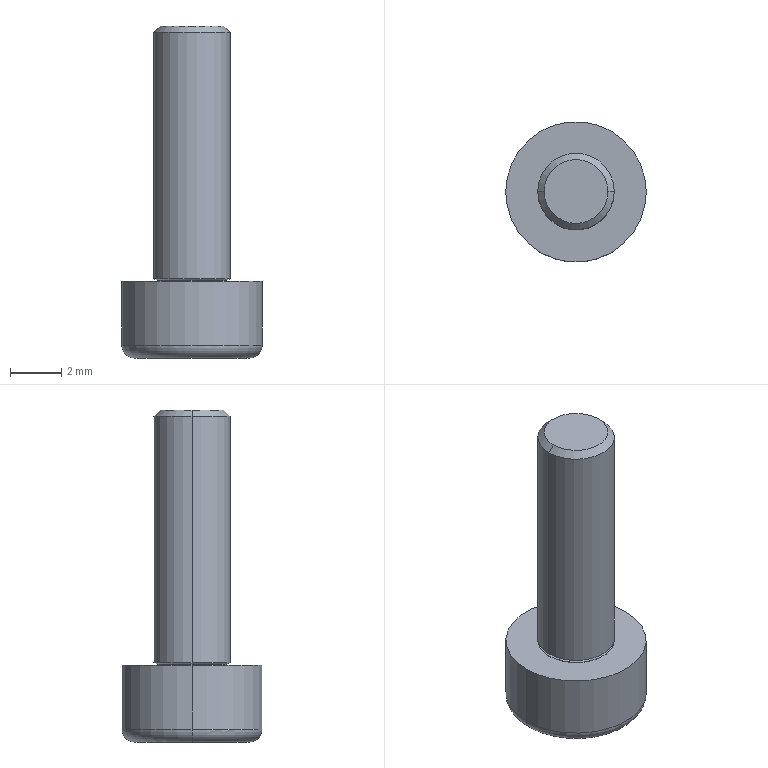Part | SolidWorks | features Attribute 1, Cut 1, Revolution 1 | 1 solid | 27 faces | box 5.5 x 5.5 x 13 mm | volume 133.94 mm3 | plane 11 | torus 6 | cylinder 6 | cone 4 | commonest cylinder face diameters 3 x4 5.5 x2
STEP:
#1=CARTESIAN_POINT('',(-1.363,0.,0.01));
#2=VERTEX_POINT('',#1);
#3=CARTESIAN_POINT('',(-1.343,0.,0.03));
#4=VERTEX_POINT('',#3);
#5=CARTESIAN_POINT('',(-1.363,0.,0.03));
#6=DIRECTION('',(0.,-1.,0.));
#7=DIRECTION('',(0.,0.,-1.));
#8=AXIS2_PLACEMENT_3D('',#5,#6,#7);
#9=CIRCLE('',#8,0.02);
#10=EDGE_CURVE('',#2,#4,#9,.T.);
#11=ORIENTED_EDGE('',*,*,#10,.T.);
#12=CARTESIAN_POINT('',(1.343,0.,0.03));
#13=VERTEX_POINT('',#12);
#14=CARTESIAN_POINT('',(0.,0.,0.03));
#15=DIRECTION('',(0.,0.,-1.));
#16=DIRECTION('',(-1.,0.,0.));
#17=AXIS2_PLACEMENT_3D('',#14,#15,#16);
#18=CIRCLE('',#17,1.343);
#19=EDGE_CURVE('',#4,#13,#18,.T.);
#20=ORIENTED_EDGE('',*,*,#19,.T.);
#21=CARTESIAN_POINT('',(1.363,0.,0.01));
#22=VERTEX_POINT('',#21);
#23=CARTESIAN_POINT('',(1.363,0.,0.03));
#24=DIRECTION('',(0.,1.,0.));
#25=DIRECTION('',(-1.,0.,0.));
#26=AXIS2_PLACEMENT_3D('',#23,#24,#25);
#27=CIRCLE('',#26,0.02);
#28=EDGE_CURVE('',#22,#13,#27,.T.);
#29=ORIENTED_EDGE('',*,*,#28,.F.);
#30=CARTESIAN_POINT('',(0.,0.,0.01));
#31=DIRECTION('',(0.,0.,-1.));
#32=DIRECTION('',(-1.,0.,0.));
#33=AXIS2_PLACEMENT_3D('',#30,#31,#32);
#34=CIRCLE('',#33,1.363);
#35=EDGE_CURVE('',#2,#22,#34,.T.);
#36=ORIENTED_EDGE('',*,*,#35,.F.);
#37=EDGE_LOOP('',(#11,#20,#29,#36));
#38=FACE_OUTER_BOUND('',#37,.T.);
#39=CARTESIAN_POINT('',(0.,0.,0.03));
#40=DIRECTION('',(0.,0.,-1.));
#41=DIRECTION('',(-1.,0.,0.));
#42=AXIS2_PLACEMENT_3D('',#39,#40,#41);
#43=TOROIDAL_SURFACE('',#42,1.363,0.02);
#44=ADVANCED_FACE('',(#38),#43,.F.);
#45=ORIENTED_EDGE('',*,*,#28,.T.);
#46=CARTESIAN_POINT('',(0.,0.,0.03));
#47=DIRECTION('',(0.,0.,-1.));
#48=DIRECTION('',(-1.,0.,0.));
#49=AXIS2_PLACEMENT_3D('',#46,#47,#48);
#50=CIRCLE('',#49,1.343);
#51=EDGE_CURVE('',#13,#4,#50,.T.);
#52=ORIENTED_EDGE('',*,*,#51,.T.);
#53=ORIENTED_EDGE('',*,*,#10,.F.);
#54=CARTESIAN_POINT('',(0.,0.,0.01));
#55=DIRECTION('',(0.,0.,-1.));
#56=DIRECTION('',(-1.,0.,0.));
#57=AXIS2_PLACEMENT_3D('',#54,#55,#56);
#58=CIRCLE('',#57,1.363);
#59=EDGE_CURVE('',#22,#2,#58,.T.);
#60=ORIENTED_EDGE('',*,*,#59,.F.);
#61=EDGE_LOOP('',(#45,#52,#53,#60));
#62=FACE_OUTER_BOUND('',#61,.T.);
#63=CARTESIAN_POINT('',(0.,0.,0.03));
#64=DIRECTION('',(0.,0.,-1.));
#65=DIRECTION('',(-1.,0.,0.));
#66=AXIS2_PLACEMENT_3D('',#63,#64,#65);
#67=TOROIDAL_SURFACE('',#66,1.363,0.02);
#68=ADVANCED_FACE('',(#62),#67,.F.);
#69=CARTESIAN_POINT('',(-1.25,0.,10.));
#70=VERTEX_POINT('',#69);
#71=CARTESIAN_POINT('',(1.25,0.,10.));
#72=VERTEX_POINT('',#71);
#73=CARTESIAN_POINT('',(0.,0.,10.));
#74=DIRECTION('',(0.,0.,-1.));
#75=DIRECTION('',(-1.,0.,0.));
#76=AXIS2_PLACEMENT_3D('',#73,#74,#75);
#77=CIRCLE('',#76,1.25);
#78=EDGE_CURVE('',#70,#72,#77,.T.);
#79=ORIENTED_EDGE('',*,*,#78,.T.);
#80=CARTESIAN_POINT('',(1.5,0.,9.75));
#81=VERTEX_POINT('',#80);
#82=CARTESIAN_POINT('',(1.25,0.,10.));
#83=DIRECTION('',(0.7071,0.,-0.7071));
#84=VECTOR('',#83,1000.);
#85=LINE('',#82,#84);
#86=EDGE_CURVE('',#72,#81,#85,.T.);
#87=ORIENTED_EDGE('',*,*,#86,.T.);
#88=CARTESIAN_POINT('',(-1.5,0.,9.75));
#89=VERTEX_POINT('',#88);
#90=CARTESIAN_POINT('',(0.,0.,9.75));
#91=DIRECTION('',(0.,0.,-1.));
#92=DIRECTION('',(-1.,0.,0.));
#93=AXIS2_PLACEMENT_3D('',#90,#91,#92);
#94=CIRCLE('',#93,1.5);
#95=EDGE_CURVE('',#89,#81,#94,.T.);
#96=ORIENTED_EDGE('',*,*,#95,.F.);
#97=CARTESIAN_POINT('',(-1.25,0.,10.));
#98=DIRECTION('',(-0.7071,0.,-0.7071));
#99=VECTOR('',#98,1000.);
#100=LINE('',#97,#99);
#101=EDGE_CURVE('',#70,#89,#100,.T.);
#102=ORIENTED_EDGE('',*,*,#101,.F.);
#103=EDGE_LOOP('',(#79,#87,#96,#102));
#104=FACE_OUTER_BOUND('',#103,.T.);
#105=CARTESIAN_POINT('',(0.,0.,10.));
#106=DIRECTION('',(0.,0.,-1.));
#107=DIRECTION('',(-1.,0.,0.));
#108=AXIS2_PLACEMENT_3D('',#105,#106,#107);
#109=CONICAL_SURFACE('',#108,1.25,0.7854);
#110=ADVANCED_FACE('',(#104),#109,.T.);
#111=ORIENTED_EDGE('',*,*,#95,.T.);
#112=CARTESIAN_POINT('',(1.5,0.,0.101));
#113=VERTEX_POINT('',#112);
#114=CARTESIAN_POINT('',(1.5,0.,-10.585));
#115=DIRECTION('',(0.,0.,-1.));
#116=VECTOR('',#115,1000.);
#117=LINE('',#114,#116);
#118=EDGE_CURVE('',#81,#113,#117,.T.);
#119=ORIENTED_EDGE('',*,*,#118,.T.);
#120=CARTESIAN_POINT('',(-1.5,0.,0.101));
#121=VERTEX_POINT('',#120);
#122=CARTESIAN_POINT('',(0.,0.,0.101));
#123=DIRECTION('',(0.,0.,-1.));
#124=DIRECTION('',(-1.,0.,0.));
#125=AXIS2_PLACEMENT_3D('',#122,#123,#124);
#126=CIRCLE('',#125,1.5);
#127=EDGE_CURVE('',#121,#113,#126,.T.);
#128=ORIENTED_EDGE('',*,*,#127,.F.);
#129=CARTESIAN_POINT('',(-1.5,0.,-10.585));
#130=DIRECTION('',(0.,0.,-1.));
#131=VECTOR('',#130,1000.);
#132=LINE('',#129,#131);
#133=EDGE_CURVE('',#89,#121,#132,.T.);
#134=ORIENTED_EDGE('',*,*,#133,.F.);
#135=EDGE_LOOP('',(#111,#119,#128,#134));
#136=FACE_OUTER_BOUND('',#135,.T.);
#137=CARTESIAN_POINT('',(0.,0.,-10.585));
#138=DIRECTION('',(0.,0.,-1.));
#139=DIRECTION('',(-1.,0.,0.));
#140=AXIS2_PLACEMENT_3D('',#137,#138,#139);
#141=CYLINDRICAL_SURFACE('',#140,1.5);
#142=ADVANCED_FACE('',(#136),#141,.T.);
#143=CARTESIAN_POINT('',(-1.357,0.,0.04879));
#144=VERTEX_POINT('',#143);
#145=CARTESIAN_POINT('',(1.357,0.,0.04879));
#146=VERTEX_POINT('',#145);
#147=CARTESIAN_POINT('',(0.,0.,0.04879));
#148=DIRECTION('',(0.,0.,-1.));
#149=DIRECTION('',(-1.,0.,0.));
#150=AXIS2_PLACEMENT_3D('',#147,#148,#149);
#151=CIRCLE('',#150,1.357);
#152=EDGE_CURVE('',#144,#146,#151,.T.);
#153=ORIENTED_EDGE('',*,*,#152,.F.);
#154=CARTESIAN_POINT('',(-1.5,0.,0.101));
#155=DIRECTION('',(-0.9397,0.,0.342));
#156=VECTOR('',#155,1000.);
#157=LINE('',#154,#156);
#158=EDGE_CURVE('',#144,#121,#157,.T.);
#159=ORIENTED_EDGE('',*,*,#158,.T.);
#160=ORIENTED_EDGE('',*,*,#127,.T.);
#161=CARTESIAN_POINT('',(1.5,0.,0.101));
#162=DIRECTION('',(0.9397,0.,0.342));
#163=VECTOR('',#162,1000.);
#164=LINE('',#161,#163);
#165=EDGE_CURVE('',#146,#113,#164,.T.);
#166=ORIENTED_EDGE('',*,*,#165,.F.);
#167=EDGE_LOOP('',(#153,#159,#160,#166));
#168=FACE_OUTER_BOUND('',#167,.T.);
#169=CARTESIAN_POINT('',(0.,0.,0.101));
#170=DIRECTION('',(0.,0.,1.));
#171=DIRECTION('',(1.,0.,0.));
#172=AXIS2_PLACEMENT_3D('',#169,#170,#171);
#173=CONICAL_SURFACE('',#172,1.5,1.222);
#174=ADVANCED_FACE('',(#168),#173,.T.);
#175=ORIENTED_EDGE('',*,*,#51,.F.);
#176=CARTESIAN_POINT('',(1.363,0.,0.03));
#177=DIRECTION('',(0.,1.,0.));
#178=DIRECTION('',(-1.,0.,0.));
#179=AXIS2_PLACEMENT_3D('',#176,#177,#178);
#180=CIRCLE('',#179,0.02);
#181=EDGE_CURVE('',#13,#146,#180,.T.);
#182=ORIENTED_EDGE('',*,*,#181,.T.);
#183=CARTESIAN_POINT('',(0.,0.,0.04879));
#184=DIRECTION('',(0.,0.,-1.));
#185=DIRECTION('',(-1.,0.,0.));
#186=AXIS2_PLACEMENT_3D('',#183,#184,#185);
#187=CIRCLE('',#186,1.357);
#188=EDGE_CURVE('',#146,#144,#187,.T.);
#189=ORIENTED_EDGE('',*,*,#188,.T.);
#190=CARTESIAN_POINT('',(-1.363,0.,0.03));
#191=DIRECTION('',(0.,-1.,0.));
#192=DIRECTION('',(0.,0.,-1.));
#193=AXIS2_PLACEMENT_3D('',#190,#191,#192);
#194=CIRCLE('',#193,0.02);
#195=EDGE_CURVE('',#4,#144,#194,.T.);
#196=ORIENTED_EDGE('',*,*,#195,.F.);
#197=EDGE_LOOP('',(#175,#182,#189,#196));
#198=FACE_OUTER_BOUND('',#197,.T.);
#199=CARTESIAN_POINT('',(0.,0.,0.03));
#200=DIRECTION('',(0.,0.,-1.));
#201=DIRECTION('',(-1.,0.,0.));
#202=AXIS2_PLACEMENT_3D('',#199,#200,#201);
#203=TOROIDAL_SURFACE('',#202,1.363,0.02);
#204=ADVANCED_FACE('',(#198),#203,.F.);
#205=CARTESIAN_POINT('',(-1.5,0.,0.01));
#206=VERTEX_POINT('',#205);
#207=CARTESIAN_POINT('',(1.5,0.,0.01));
#208=VERTEX_POINT('',#207);
#209=CARTESIAN_POINT('',(0.,0.,0.01));
#210=DIRECTION('',(0.,0.,-1.));
#211=DIRECTION('',(-1.,0.,0.));
#212=AXIS2_PLACEMENT_3D('',#209,#210,#211);
#213=CIRCLE('',#212,1.5);
#214=EDGE_CURVE('',#206,#208,#213,.T.);
#215=ORIENTED_EDGE('',*,*,#214,.T.);
#216=CARTESIAN_POINT('',(1.5,0.,0.));
#217=VERTEX_POINT('',#216);
#218=CARTESIAN_POINT('',(1.5,0.,-10.585));
#219=DIRECTION('',(0.,0.,-1.));
#220=VECTOR('',#219,1000.);
#221=LINE('',#218,#220);
#222=EDGE_CURVE('',#208,#217,#221,.T.);
#223=ORIENTED_EDGE('',*,*,#222,.T.);
#224=CARTESIAN_POINT('',(-1.5,0.,0.));
#225=VERTEX_POINT('',#224);
#226=CARTESIAN_POINT('',(0.,0.,0.));
#227=DIRECTION('',(0.,0.,-1.));
#228=DIRECTION('',(-1.,0.,0.));
#229=AXIS2_PLACEMENT_3D('',#226,#227,#228);
#230=CIRCLE('',#229,1.5);
#231=EDGE_CURVE('',#225,#217,#230,.T.);
#232=ORIENTED_EDGE('',*,*,#231,.F.);
#233=CARTESIAN_POINT('',(-1.5,0.,-10.585));
#234=DIRECTION('',(0.,0.,-1.));
#235=VECTOR('',#234,1000.);
#236=LINE('',#233,#235);
#237=EDGE_CURVE('',#206,#225,#236,.T.);
#238=ORIENTED_EDGE('',*,*,#237,.F.);
#239=EDGE_LOOP('',(#215,#223,#232,#238));
#240=FACE_OUTER_BOUND('',#239,.T.);
#241=CARTESIAN_POINT('',(0.,0.,-10.585));
#242=DIRECTION('',(0.,0.,-1.));
#243=DIRECTION('',(-1.,0.,0.));
#244=AXIS2_PLACEMENT_3D('',#241,#242,#243);
#245=CYLINDRICAL_SURFACE('',#244,1.5);
#246=ADVANCED_FACE('',(#240),#245,.T.);
#247=CARTESIAN_POINT('',(-2.75,0.,0.));
#248=VERTEX_POINT('',#247);
#249=CARTESIAN_POINT('',(2.75,0.,0.));
#250=VERTEX_POINT('',#249);
#251=CARTESIAN_POINT('',(0.,0.,0.));
#252=DIRECTION('',(0.,0.,-1.));
#253=DIRECTION('',(-1.,0.,0.));
#254=AXIS2_PLACEMENT_3D('',#251,#252,#253);
#255=CIRCLE('',#254,2.75);
#256=EDGE_CURVE('',#248,#250,#255,.T.);
#257=ORIENTED_EDGE('',*,*,#256,.T.);
#258=CARTESIAN_POINT('',(2.75,0.,-2.5));
#259=VERTEX_POINT('',#258);
#260=CARTESIAN_POINT('',(2.75,0.,-10.585));
#261=DIRECTION('',(0.,0.,-1.));
#262=VECTOR('',#261,1000.);
#263=LINE('',#260,#262);
#264=EDGE_CURVE('',#250,#259,#263,.T.);
#265=ORIENTED_EDGE('',*,*,#264,.T.);
#266=CARTESIAN_POINT('',(-2.75,0.,-2.5));
#267=VERTEX_POINT('',#266);
#268=CARTESIAN_POINT('',(0.,0.,-2.5));
#269=DIRECTION('',(0.,0.,-1.));
#270=DIRECTION('',(-1.,0.,0.));
#271=AXIS2_PLACEMENT_3D('',#268,#269,#270);
#272=CIRCLE('',#271,2.75);
#273=EDGE_CURVE('',#267,#259,#272,.T.);
#274=ORIENTED_EDGE('',*,*,#273,.F.);
#275=CARTESIAN_POINT('',(-2.75,0.,-10.585));
#276=DIRECTION('',(0.,0.,-1.));
#277=VECTOR('',#276,1000.);
#278=LINE('',#275,#277);
#279=EDGE_CURVE('',#248,#267,#278,.T.);
#280=ORIENTED_EDGE('',*,*,#279,.F.);
#281=EDGE_LOOP('',(#257,#265,#274,#280));
#282=FACE_OUTER_BOUND('',#281,.T.);
#283=CARTESIAN_POINT('',(0.,0.,-10.585));
#284=DIRECTION('',(0.,0.,-1.));
#285=DIRECTION('',(-1.,0.,0.));
#286=AXIS2_PLACEMENT_3D('',#283,#284,#285);
#287=CYLINDRICAL_SURFACE('',#286,2.75);
#288=ADVANCED_FACE('',(#282),#287,.T.);
#289=ORIENTED_EDGE('',*,*,#273,.T.);
#290=CARTESIAN_POINT('',(2.25,0.,-3.));
#291=VERTEX_POINT('',#290);
#292=CARTESIAN_POINT('',(2.25,0.,-2.5));
#293=DIRECTION('',(0.,1.,0.));
#294=DIRECTION('',(-1.,0.,0.));
#295=AXIS2_PLACEMENT_3D('',#292,#293,#294);
#296=CIRCLE('',#295,0.5);
#297=EDGE_CURVE('',#259,#291,#296,.T.);
#298=ORIENTED_EDGE('',*,*,#297,.T.);
#299=CARTESIAN_POINT('',(-2.25,0.,-3.));
#300=VERTEX_POINT('',#299);
#301=CARTESIAN_POINT('',(0.,0.,-3.));
#302=DIRECTION('',(0.,0.,-1.));
#303=DIRECTION('',(-1.,0.,0.));
#304=AXIS2_PLACEMENT_3D('',#301,#302,#303);
#305=CIRCLE('',#304,2.25);
#306=EDGE_CURVE('',#300,#291,#305,.T.);
#307=ORIENTED_EDGE('',*,*,#306,.F.);
#308=CARTESIAN_POINT('',(-2.25,0.,-2.5));
#309=DIRECTION('',(0.,-1.,0.));
#310=DIRECTION('',(0.,0.,-1.));
#311=AXIS2_PLACEMENT_3D('',#308,#309,#310);
#312=CIRCLE('',#311,0.5);
#313=EDGE_CURVE('',#267,#300,#312,.T.);
#314=ORIENTED_EDGE('',*,*,#313,.F.);
#315=EDGE_LOOP('',(#289,#298,#307,#314));
#316=FACE_OUTER_BOUND('',#315,.T.);
#317=CARTESIAN_POINT('',(0.,0.,-2.5));
#318=DIRECTION('',(0.,0.,-1.));
#319=DIRECTION('',(-1.,0.,0.));
#320=AXIS2_PLACEMENT_3D('',#317,#318,#319);
#321=TOROIDAL_SURFACE('',#320,2.25,0.5);
#322=ADVANCED_FACE('',(#316),#321,.T.);
#323=ORIENTED_EDGE('',*,*,#297,.F.);
#324=CARTESIAN_POINT('',(0.,0.,-2.5));
#325=DIRECTION('',(0.,0.,-1.));
#326=DIRECTION('',(-1.,0.,0.));
#327=AXIS2_PLACEMENT_3D('',#324,#325,#326);
#328=CIRCLE('',#327,2.75);
#329=EDGE_CURVE('',#259,#267,#328,.T.);
#330=ORIENTED_EDGE('',*,*,#329,.T.);
#331=ORIENTED_EDGE('',*,*,#313,.T.);
#332=CARTESIAN_POINT('',(0.,0.,-3.));
#333=DIRECTION('',(0.,0.,-1.));
#334=DIRECTION('',(-1.,0.,0.));
#335=AXIS2_PLACEMENT_3D('',#332,#333,#334);
#336=CIRCLE('',#335,2.25);
#337=EDGE_CURVE('',#291,#300,#336,.T.);
#338=ORIENTED_EDGE('',*,*,#337,.F.);
#339=EDGE_LOOP('',(#323,#330,#331,#338));
#340=FACE_OUTER_BOUND('',#339,.T.);
#341=CARTESIAN_POINT('',(0.,0.,-2.5));
#342=DIRECTION('',(0.,0.,-1.));
#343=DIRECTION('',(-1.,0.,0.));
#344=AXIS2_PLACEMENT_3D('',#341,#342,#343);
#345=TOROIDAL_SURFACE('',#344,2.25,0.5);
#346=ADVANCED_FACE('',(#340),#345,.T.);
#347=ORIENTED_EDGE('',*,*,#264,.F.);
#348=CARTESIAN_POINT('',(0.,0.,0.));
#349=DIRECTION('',(0.,0.,-1.));
#350=DIRECTION('',(-1.,0.,0.));
#351=AXIS2_PLACEMENT_3D('',#348,#349,#350);
#352=CIRCLE('',#351,2.75);
#353=EDGE_CURVE('',#250,#248,#352,.T.);
#354=ORIENTED_EDGE('',*,*,#353,.T.);
#355=ORIENTED_EDGE('',*,*,#279,.T.);
#356=ORIENTED_EDGE('',*,*,#329,.F.);
#357=EDGE_LOOP('',(#347,#354,#355,#356));
#358=FACE_OUTER_BOUND('',#357,.T.);
#359=CARTESIAN_POINT('',(0.,0.,-10.585));
#360=DIRECTION('',(0.,0.,-1.));
#361=DIRECTION('',(-1.,0.,0.));
#362=AXIS2_PLACEMENT_3D('',#359,#360,#361);
#363=CYLINDRICAL_SURFACE('',#362,2.75);
#364=ADVANCED_FACE('',(#358),#363,.T.);
#365=ORIENTED_EDGE('',*,*,#256,.F.);
#366=ORIENTED_EDGE('',*,*,#353,.F.);
#367=EDGE_LOOP('',(#365,#366));
#368=FACE_OUTER_BOUND('',#367,.T.);
#369=ORIENTED_EDGE('',*,*,#231,.T.);
#370=CARTESIAN_POINT('',(0.,0.,0.));
#371=DIRECTION('',(0.,0.,-1.));
#372=DIRECTION('',(-1.,0.,0.));
#373=AXIS2_PLACEMENT_3D('',#370,#371,#372);
#374=CIRCLE('',#373,1.5);
#375=EDGE_CURVE('',#217,#225,#374,.T.);
#376=ORIENTED_EDGE('',*,*,#375,.T.);
#377=EDGE_LOOP('',(#369,#376));
#378=FACE_BOUND('',#377,.T.);
#379=CARTESIAN_POINT('',(-2.75,0.,0.));
#380=DIRECTION('',(0.,0.,-1.));
#381=DIRECTION('',(-1.,0.,0.));
#382=AXIS2_PLACEMENT_3D('',#379,#380,#381);
#383=PLANE('',#382);
#384=ADVANCED_FACE('',(#368,#378),#383,.F.);
#385=ORIENTED_EDGE('',*,*,#222,.F.);
#386=CARTESIAN_POINT('',(0.,0.,0.01));
#387=DIRECTION('',(0.,0.,-1.));
#388=DIRECTION('',(-1.,0.,0.));
#389=AXIS2_PLACEMENT_3D('',#386,#387,#388);
#390=CIRCLE('',#389,1.5);
#391=EDGE_CURVE('',#208,#206,#390,.T.);
#392=ORIENTED_EDGE('',*,*,#391,.T.);
#393=ORIENTED_EDGE('',*,*,#237,.T.);
#394=ORIENTED_EDGE('',*,*,#375,.F.);
#395=EDGE_LOOP('',(#385,#392,#393,#394));
#396=FACE_OUTER_BOUND('',#395,.T.);
#397=CARTESIAN_POINT('',(0.,0.,-10.585));
#398=DIRECTION('',(0.,0.,-1.));
#399=DIRECTION('',(-1.,0.,0.));
#400=AXIS2_PLACEMENT_3D('',#397,#398,#399);
#401=CYLINDRICAL_SURFACE('',#400,1.5);
#402=ADVANCED_FACE('',(#396),#401,.T.);
#403=ORIENTED_EDGE('',*,*,#214,.F.);
#404=ORIENTED_EDGE('',*,*,#391,.F.);
#405=EDGE_LOOP('',(#403,#404));
#406=FACE_OUTER_BOUND('',#405,.T.);
#407=ORIENTED_EDGE('',*,*,#35,.T.);
#408=ORIENTED_EDGE('',*,*,#59,.T.);
#409=EDGE_LOOP('',(#407,#408));
#410=FACE_BOUND('',#409,.T.);
#411=CARTESIAN_POINT('',(-1.5,0.,0.01));
#412=DIRECTION('',(0.,0.,-1.));
#413=DIRECTION('',(-1.,0.,0.));
#414=AXIS2_PLACEMENT_3D('',#411,#412,#413);
#415=PLANE('',#414);
#416=ADVANCED_FACE('',(#406,#410),#415,.F.);
#417=ORIENTED_EDGE('',*,*,#19,.F.);
#418=ORIENTED_EDGE('',*,*,#195,.T.);
#419=ORIENTED_EDGE('',*,*,#152,.T.);
#420=ORIENTED_EDGE('',*,*,#181,.F.);
#421=EDGE_LOOP('',(#417,#418,#419,#420));
#422=FACE_OUTER_BOUND('',#421,.T.);
#423=CARTESIAN_POINT('',(0.,0.,0.03));
#424=DIRECTION('',(0.,0.,-1.));
#425=DIRECTION('',(-1.,0.,0.));
#426=AXIS2_PLACEMENT_3D('',#423,#424,#425);
#427=TOROIDAL_SURFACE('',#426,1.363,0.02);
#428=ADVANCED_FACE('',(#422),#427,.F.);
#429=ORIENTED_EDGE('',*,*,#158,.F.);
#430=ORIENTED_EDGE('',*,*,#188,.F.);
#431=ORIENTED_EDGE('',*,*,#165,.T.);
#432=CARTESIAN_POINT('',(0.,0.,0.101));
#433=DIRECTION('',(0.,0.,-1.));
#434=DIRECTION('',(-1.,0.,0.));
#435=AXIS2_PLACEMENT_3D('',#432,#433,#434);
#436=CIRCLE('',#435,1.5);
#437=EDGE_CURVE('',#113,#121,#436,.T.);
#438=ORIENTED_EDGE('',*,*,#437,.T.);
#439=EDGE_LOOP('',(#429,#430,#431,#438));
#440=FACE_OUTER_BOUND('',#439,.T.);
#441=CARTESIAN_POINT('',(0.,0.,0.101));
#442=DIRECTION('',(0.,0.,1.));
#443=DIRECTION('',(1.,0.,0.));
#444=AXIS2_PLACEMENT_3D('',#441,#442,#443);
#445=CONICAL_SURFACE('',#444,1.5,1.222);
#446=ADVANCED_FACE('',(#440),#445,.T.);
#447=ORIENTED_EDGE('',*,*,#118,.F.);
#448=CARTESIAN_POINT('',(0.,0.,9.75));
#449=DIRECTION('',(0.,0.,-1.));
#450=DIRECTION('',(-1.,0.,0.));
#451=AXIS2_PLACEMENT_3D('',#448,#449,#450);
#452=CIRCLE('',#451,1.5);
#453=EDGE_CURVE('',#81,#89,#452,.T.);
#454=ORIENTED_EDGE('',*,*,#453,.T.);
#455=ORIENTED_EDGE('',*,*,#133,.T.);
#456=ORIENTED_EDGE('',*,*,#437,.F.);
#457=EDGE_LOOP('',(#447,#454,#455,#456));
#458=FACE_OUTER_BOUND('',#457,.T.);
#459=CARTESIAN_POINT('',(0.,0.,-10.585));
#460=DIRECTION('',(0.,0.,-1.));
#461=DIRECTION('',(-1.,0.,0.));
#462=AXIS2_PLACEMENT_3D('',#459,#460,#461);
#463=CYLINDRICAL_SURFACE('',#462,1.5);
#464=ADVANCED_FACE('',(#458),#463,.T.);
#465=ORIENTED_EDGE('',*,*,#86,.F.);
#466=CARTESIAN_POINT('',(0.,0.,10.));
#467=DIRECTION('',(0.,0.,-1.));
#468=DIRECTION('',(-1.,0.,0.));
#469=AXIS2_PLACEMENT_3D('',#466,#467,#468);
#470=CIRCLE('',#469,1.25);
#471=EDGE_CURVE('',#72,#70,#470,.T.);
#472=ORIENTED_EDGE('',*,*,#471,.T.);
#473=ORIENTED_EDGE('',*,*,#101,.T.);
#474=ORIENTED_EDGE('',*,*,#453,.F.);
#475=EDGE_LOOP('',(#465,#472,#473,#474));
#476=FACE_OUTER_BOUND('',#475,.T.);
#477=CARTESIAN_POINT('',(0.,0.,10.));
#478=DIRECTION('',(0.,0.,-1.));
#479=DIRECTION('',(-1.,0.,0.));
#480=AXIS2_PLACEMENT_3D('',#477,#478,#479);
#481=CONICAL_SURFACE('',#480,1.25,0.7854);
#482=ADVANCED_FACE('',(#476),#481,.T.);
#483=ORIENTED_EDGE('',*,*,#78,.F.);
#484=ORIENTED_EDGE('',*,*,#471,.F.);
#485=EDGE_LOOP('',(#483,#484));
#486=FACE_OUTER_BOUND('',#485,.T.);
#487=CARTESIAN_POINT('',(-1.25,0.,10.));
#488=DIRECTION('',(0.,0.,-1.));
#489=DIRECTION('',(-1.,0.,0.));
#490=AXIS2_PLACEMENT_3D('',#487,#488,#489);
#491=PLANE('',#490);
#492=ADVANCED_FACE('',(#486),#491,.F.);
#493=CARTESIAN_POINT('',(1.443,0.,-3.));
#494=VERTEX_POINT('',#493);
#495=CARTESIAN_POINT('',(0.7217,-1.25,-3.));
#496=VERTEX_POINT('',#495);
#497=CARTESIAN_POINT('',(1.443,0.,-3.));
#498=DIRECTION('',(-0.5,-0.866,0.));
#499=VECTOR('',#498,1000.);
#500=LINE('',#497,#499);
#501=EDGE_CURVE('',#494,#496,#500,.T.);
#502=ORIENTED_EDGE('',*,*,#501,.F.);
#503=CARTESIAN_POINT('',(0.7217,1.25,-3.));
#504=VERTEX_POINT('',#503);
#505=CARTESIAN_POINT('',(0.7217,1.25,-3.));
#506=DIRECTION('',(0.5,-0.866,0.));
#507=VECTOR('',#506,1000.);
#508=LINE('',#505,#507);
#509=EDGE_CURVE('',#504,#494,#508,.T.);
#510=ORIENTED_EDGE('',*,*,#509,.F.);
#511=CARTESIAN_POINT('',(-0.7217,1.25,-3.));
#512=VERTEX_POINT('',#511);
#513=CARTESIAN_POINT('',(-0.7217,1.25,-3.));
#514=DIRECTION('',(1.,0.,0.));
#515=VECTOR('',#514,1000.);
#516=LINE('',#513,#515);
#517=EDGE_CURVE('',#512,#504,#516,.T.);
#518=ORIENTED_EDGE('',*,*,#517,.F.);
#519=CARTESIAN_POINT('',(-1.443,0.,-3.));
#520=VERTEX_POINT('',#519);
#521=CARTESIAN_POINT('',(-1.443,0.,-3.));
#522=DIRECTION('',(0.5,0.866,0.));
#523=VECTOR('',#522,1000.);
#524=LINE('',#521,#523);
#525=EDGE_CURVE('',#520,#512,#524,.T.);
#526=ORIENTED_EDGE('',*,*,#525,.F.);
#527=CARTESIAN_POINT('',(-0.7217,-1.25,-3.));
#528=VERTEX_POINT('',#527);
#529=CARTESIAN_POINT('',(-0.7217,-1.25,-3.));
#530=DIRECTION('',(-0.5,0.866,0.));
#531=VECTOR('',#530,1000.);
#532=LINE('',#529,#531);
#533=EDGE_CURVE('',#528,#520,#532,.T.);
#534=ORIENTED_EDGE('',*,*,#533,.F.);
#535=CARTESIAN_POINT('',(0.7217,-1.25,-3.));
#536=DIRECTION('',(-1.,0.,0.));
#537=VECTOR('',#536,1000.);
#538=LINE('',#535,#537);
#539=EDGE_CURVE('',#496,#528,#538,.T.);
#540=ORIENTED_EDGE('',*,*,#539,.F.);
#541=EDGE_LOOP('',(#502,#510,#518,#526,#534,#540));
#542=FACE_BOUND('',#541,.T.);
#543=ORIENTED_EDGE('',*,*,#306,.T.);
#544=ORIENTED_EDGE('',*,*,#337,.T.);
#545=EDGE_LOOP('',(#543,#544));
#546=FACE_OUTER_BOUND('',#545,.T.);
#547=CARTESIAN_POINT('',(0.,0.,-3.));
#548=DIRECTION('',(0.,0.,1.));
#549=DIRECTION('',(1.,0.,0.));
#550=AXIS2_PLACEMENT_3D('',#547,#548,#549);
#551=PLANE('',#550);
#552=ADVANCED_FACE('',(#542,#546),#551,.F.);
#553=ORIENTED_EDGE('',*,*,#509,.T.);
#554=CARTESIAN_POINT('',(1.443,0.,-1.75));
#555=VERTEX_POINT('',#554);
#556=CARTESIAN_POINT('',(1.443,0.,-1.75));
#557=DIRECTION('',(0.,0.,-1.));
#558=VECTOR('',#557,1000.);
#559=LINE('',#556,#558);
#560=EDGE_CURVE('',#555,#494,#559,.T.);
#561=ORIENTED_EDGE('',*,*,#560,.F.);
#562=CARTESIAN_POINT('',(0.7217,1.25,-1.75));
#563=VERTEX_POINT('',#562);
#564=CARTESIAN_POINT('',(0.7217,1.25,-1.75));
#565=DIRECTION('',(0.5,-0.866,0.));
#566=VECTOR('',#565,1000.);
#567=LINE('',#564,#566);
#568=EDGE_CURVE('',#563,#555,#567,.T.);
#569=ORIENTED_EDGE('',*,*,#568,.F.);
#570=CARTESIAN_POINT('',(0.7217,1.25,-1.75));
#571=DIRECTION('',(0.,0.,-1.));
#572=VECTOR('',#571,1000.);
#573=LINE('',#570,#572);
#574=EDGE_CURVE('',#563,#504,#573,.T.);
#575=ORIENTED_EDGE('',*,*,#574,.T.);
#576=EDGE_LOOP('',(#553,#561,#569,#575));
#577=FACE_OUTER_BOUND('',#576,.T.);
#578=CARTESIAN_POINT('',(0.7217,1.25,-1.75));
#579=DIRECTION('',(0.866,0.5,0.));
#580=DIRECTION('',(-0.5,0.866,0.));
#581=AXIS2_PLACEMENT_3D('',#578,#579,#580);
#582=PLANE('',#581);
#583=ADVANCED_FACE('',(#577),#582,.F.);
#584=ORIENTED_EDGE('',*,*,#517,.T.);
#585=ORIENTED_EDGE('',*,*,#574,.F.);
#586=CARTESIAN_POINT('',(-0.7217,1.25,-1.75));
#587=VERTEX_POINT('',#586);
#588=CARTESIAN_POINT('',(-0.7217,1.25,-1.75));
#589=DIRECTION('',(1.,0.,0.));
#590=VECTOR('',#589,1000.);
#591=LINE('',#588,#590);
#592=EDGE_CURVE('',#587,#563,#591,.T.);
#593=ORIENTED_EDGE('',*,*,#592,.F.);
#594=CARTESIAN_POINT('',(-0.7217,1.25,-1.75));
#595=DIRECTION('',(0.,0.,-1.));
#596=VECTOR('',#595,1000.);
#597=LINE('',#594,#596);
#598=EDGE_CURVE('',#587,#512,#597,.T.);
#599=ORIENTED_EDGE('',*,*,#598,.T.);
#600=EDGE_LOOP('',(#584,#585,#593,#599));
#601=FACE_OUTER_BOUND('',#600,.T.);
#602=CARTESIAN_POINT('',(-0.7217,1.25,-1.75));
#603=DIRECTION('',(0.,1.,0.));
#604=DIRECTION('',(0.,0.,1.));
#605=AXIS2_PLACEMENT_3D('',#602,#603,#604);
#606=PLANE('',#605);
#607=ADVANCED_FACE('',(#601),#606,.F.);
#608=ORIENTED_EDGE('',*,*,#525,.T.);
#609=ORIENTED_EDGE('',*,*,#598,.F.);
#610=CARTESIAN_POINT('',(-1.443,0.,-1.75));
#611=VERTEX_POINT('',#610);
#612=CARTESIAN_POINT('',(-1.443,0.,-1.75));
#613=DIRECTION('',(0.5,0.866,0.));
#614=VECTOR('',#613,1000.);
#615=LINE('',#612,#614);
#616=EDGE_CURVE('',#611,#587,#615,.T.);
#617=ORIENTED_EDGE('',*,*,#616,.F.);
#618=CARTESIAN_POINT('',(-1.443,0.,-1.75));
#619=DIRECTION('',(0.,0.,-1.));
#620=VECTOR('',#619,1000.);
#621=LINE('',#618,#620);
#622=EDGE_CURVE('',#611,#520,#621,.T.);
#623=ORIENTED_EDGE('',*,*,#622,.T.);
#624=EDGE_LOOP('',(#608,#609,#617,#623));
#625=FACE_OUTER_BOUND('',#624,.T.);
#626=CARTESIAN_POINT('',(-1.443,0.,-1.75));
#627=DIRECTION('',(-0.866,0.5,0.));
#628=DIRECTION('',(-0.5,-0.866,0.));
#629=AXIS2_PLACEMENT_3D('',#626,#627,#628);
#630=PLANE('',#629);
#631=ADVANCED_FACE('',(#625),#630,.F.);
#632=ORIENTED_EDGE('',*,*,#533,.T.);
#633=ORIENTED_EDGE('',*,*,#622,.F.);
#634=CARTESIAN_POINT('',(-0.7217,-1.25,-1.75));
#635=VERTEX_POINT('',#634);
#636=CARTESIAN_POINT('',(-0.7217,-1.25,-1.75));
#637=DIRECTION('',(-0.5,0.866,0.));
#638=VECTOR('',#637,1000.);
#639=LINE('',#636,#638);
#640=EDGE_CURVE('',#635,#611,#639,.T.);
#641=ORIENTED_EDGE('',*,*,#640,.F.);
#642=CARTESIAN_POINT('',(-0.7217,-1.25,-1.75));
#643=DIRECTION('',(0.,0.,-1.));
#644=VECTOR('',#643,1000.);
#645=LINE('',#642,#644);
#646=EDGE_CURVE('',#635,#528,#645,.T.);
#647=ORIENTED_EDGE('',*,*,#646,.T.);
#648=EDGE_LOOP('',(#632,#633,#641,#647));
#649=FACE_OUTER_BOUND('',#648,.T.);
#650=CARTESIAN_POINT('',(-0.7217,-1.25,-1.75));
#651=DIRECTION('',(-0.866,-0.5,0.));
#652=DIRECTION('',(0.5,-0.866,0.));
#653=AXIS2_PLACEMENT_3D('',#650,#651,#652);
#654=PLANE('',#653);
#655=ADVANCED_FACE('',(#649),#654,.F.);
#656=ORIENTED_EDGE('',*,*,#539,.T.);
#657=ORIENTED_EDGE('',*,*,#646,.F.);
#658=CARTESIAN_POINT('',(0.7217,-1.25,-1.75));
#659=VERTEX_POINT('',#658);
#660=CARTESIAN_POINT('',(0.7217,-1.25,-1.75));
#661=DIRECTION('',(-1.,0.,0.));
#662=VECTOR('',#661,1000.);
#663=LINE('',#660,#662);
#664=EDGE_CURVE('',#659,#635,#663,.T.);
#665=ORIENTED_EDGE('',*,*,#664,.F.);
#666=CARTESIAN_POINT('',(0.7217,-1.25,-1.75));
#667=DIRECTION('',(0.,0.,-1.));
#668=VECTOR('',#667,1000.);
#669=LINE('',#666,#668);
#670=EDGE_CURVE('',#659,#496,#669,.T.);
#671=ORIENTED_EDGE('',*,*,#670,.T.);
#672=EDGE_LOOP('',(#656,#657,#665,#671));
#673=FACE_OUTER_BOUND('',#672,.T.);
#674=CARTESIAN_POINT('',(0.7217,-1.25,-1.75));
#675=DIRECTION('',(0.,-1.,0.));
#676=DIRECTION('',(0.,0.,-1.));
#677=AXIS2_PLACEMENT_3D('',#674,#675,#676);
#678=PLANE('',#677);
#679=ADVANCED_FACE('',(#673),#678,.F.);
#680=ORIENTED_EDGE('',*,*,#501,.T.);
#681=ORIENTED_EDGE('',*,*,#670,.F.);
#682=CARTESIAN_POINT('',(1.443,0.,-1.75));
#683=DIRECTION('',(-0.5,-0.866,0.));
#684=VECTOR('',#683,1000.);
#685=LINE('',#682,#684);
#686=EDGE_CURVE('',#555,#659,#685,.T.);
#687=ORIENTED_EDGE('',*,*,#686,.F.);
#688=ORIENTED_EDGE('',*,*,#560,.T.);
#689=EDGE_LOOP('',(#680,#681,#687,#688));
#690=FACE_OUTER_BOUND('',#689,.T.);
#691=CARTESIAN_POINT('',(1.443,0.,-1.75));
#692=DIRECTION('',(0.866,-0.5,0.));
#693=DIRECTION('',(0.5,0.866,0.));
#694=AXIS2_PLACEMENT_3D('',#691,#692,#693);
#695=PLANE('',#694);
#696=ADVANCED_FACE('',(#690),#695,.F.);
#697=ORIENTED_EDGE('',*,*,#568,.T.);
#698=ORIENTED_EDGE('',*,*,#686,.T.);
#699=ORIENTED_EDGE('',*,*,#664,.T.);
#700=ORIENTED_EDGE('',*,*,#640,.T.);
#701=ORIENTED_EDGE('',*,*,#616,.T.);
#702=ORIENTED_EDGE('',*,*,#592,.T.);
#703=EDGE_LOOP('',(#697,#698,#699,#700,#701,#702));
#704=FACE_OUTER_BOUND('',#703,.T.);
#705=CARTESIAN_POINT('',(1.443,0.,-1.75));
#706=DIRECTION('',(0.,0.,-1.));
#707=DIRECTION('',(-1.,0.,0.));
#708=AXIS2_PLACEMENT_3D('',#705,#706,#707);
#709=PLANE('',#708);
#710=ADVANCED_FACE('',(#704),#709,.T.);
#711=CLOSED_SHELL('',(#44,#68,#110,#142,#174,#204,#246,#288,#322,#346,#364,#384,#402,#416,#428,#446,#464,#482,#492,#552,#583,#607,#631,#655,#679,#696,#710));
#712=MANIFOLD_SOLID_BREP('',#711);
#713=CARTESIAN_POINT('',(0.,0.,0.));
#714=DIRECTION('',(0.,0.,1.));
#715=DIRECTION('',(1.,0.,0.));
#716=AXIS2_PLACEMENT_3D('',#713,#714,#715);
#717=(LENGTH_UNIT()NAMED_UNIT(*)SI_UNIT(.MILLI.,.METRE.));
#718=UNCERTAINTY_MEASURE_WITH_UNIT(LENGTH_MEASURE(0.00001),#717,'','');
#719=(NAMED_UNIT(*)PLANE_ANGLE_UNIT()SI_UNIT($,.RADIAN.));
#720=(NAMED_UNIT(*)SI_UNIT($,.STERADIAN.)SOLID_ANGLE_UNIT());
#721=(GEOMETRIC_REPRESENTATION_CONTEXT(3)GLOBAL_UNCERTAINTY_ASSIGNED_CONTEXT((#718))GLOBAL_UNIT_ASSIGNED_CONTEXT((#717,#719,#720))REPRESENTATION_CONTEXT('',''));
#722=ADVANCED_BREP_SHAPE_REPRESENTATION('',(#712,#716),#721);